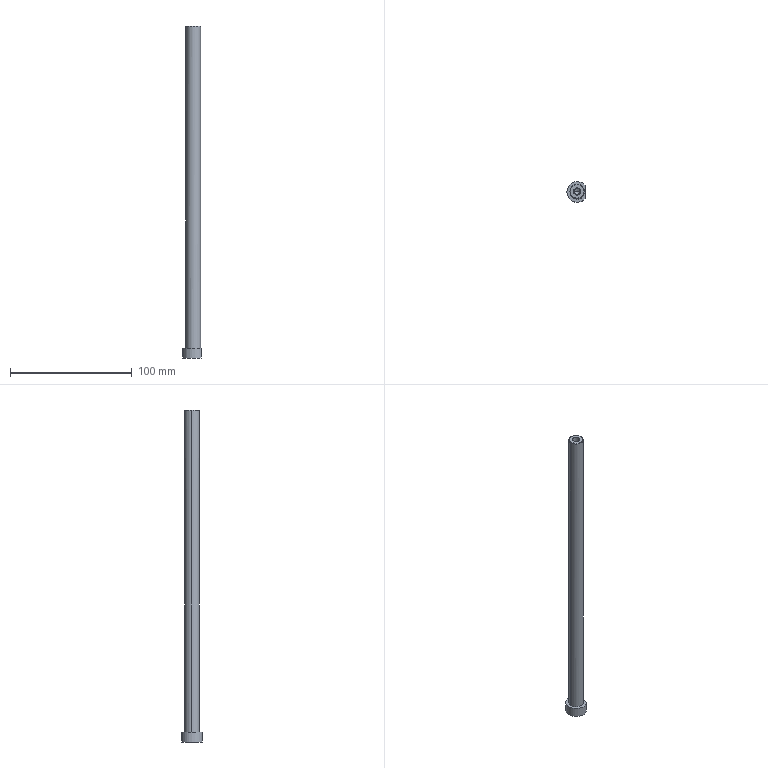Part | Creo | 1 solid | 16 faces | box 15 x 17 x 272.628 mm | volume 31426 mm3 | cylinder 7 | plane 5 | cone 4 | commonest cylinder face diameters 5 x2 6 x2 12 x2 17 x1
STEP:
#1=CARTESIAN_POINT('',(31.5,-23.477,-288.));
#2=VERTEX_POINT('',#1);
#3=CARTESIAN_POINT('',(31.5,-12.523,-288.));
#4=VERTEX_POINT('',#3);
#5=CARTESIAN_POINT('',(31.5,-23.477,-288.));
#6=DIRECTION('',(0.,1.,0.));
#7=VECTOR('',#6,10.954);
#8=LINE('',#5,#7);
#9=EDGE_CURVE('',#2,#4,#8,.T.);
#10=ORIENTED_EDGE('',*,*,#9,.F.);
#11=CARTESIAN_POINT('',(25.,-18.,-288.));
#12=DIRECTION('',(0.,0.,1.));
#13=DIRECTION('',(0.7647,0.6444,0.));
#14=AXIS2_PLACEMENT_3D('',#11,#12,#13);
#15=CIRCLE('',#14,8.5);
#16=EDGE_CURVE('',#4,#2,#15,.T.);
#17=ORIENTED_EDGE('',*,*,#16,.F.);
#18=EDGE_LOOP('',(#10,#17));
#19=FACE_OUTER_BOUND('',#18,.F.);
#20=CARTESIAN_POINT('',(19.,-18.,-288.));
#21=VERTEX_POINT('',#20);
#22=CARTESIAN_POINT('',(31.,-18.,-288.));
#23=VERTEX_POINT('',#22);
#24=CARTESIAN_POINT('',(25.,-18.,-288.));
#25=DIRECTION('',(0.,0.,-1.));
#26=DIRECTION('',(-1.,0.,0.));
#27=AXIS2_PLACEMENT_3D('',#24,#25,#26);
#28=CIRCLE('',#27,6.);
#29=EDGE_CURVE('',#21,#23,#28,.T.);
#30=ORIENTED_EDGE('',*,*,#29,.F.);
#31=CARTESIAN_POINT('',(25.,-18.,-288.));
#32=DIRECTION('',(0.,0.,-1.));
#33=DIRECTION('',(1.,0.,0.));
#34=AXIS2_PLACEMENT_3D('',#31,#32,#33);
#35=CIRCLE('',#34,6.);
#36=EDGE_CURVE('',#23,#21,#35,.T.);
#37=ORIENTED_EDGE('',*,*,#36,.F.);
#38=EDGE_LOOP('',(#30,#37));
#39=FACE_BOUND('',#38,.F.);
#40=CARTESIAN_POINT('',(25.,-18.,-288.));
#41=DIRECTION('',(0.,0.,1.));
#42=DIRECTION('',(-1.,0.,0.));
#43=AXIS2_PLACEMENT_3D('',#40,#41,#42);
#44=PLANE('',#43);
#45=ADVANCED_FACE('',(#19,#39),#44,.T.);
#46=CARTESIAN_POINT('',(31.5,-23.477,-296.));
#47=VERTEX_POINT('',#46);
#48=CARTESIAN_POINT('',(31.5,-23.477,-296.));
#49=DIRECTION('',(0.,0.,1.));
#50=VECTOR('',#49,8.);
#51=LINE('',#48,#50);
#52=EDGE_CURVE('',#47,#2,#51,.T.);
#53=ORIENTED_EDGE('',*,*,#52,.T.);
#54=ORIENTED_EDGE('',*,*,#9,.T.);
#55=CARTESIAN_POINT('',(31.5,-12.523,-296.));
#56=VERTEX_POINT('',#55);
#57=CARTESIAN_POINT('',(31.5,-12.523,-288.));
#58=DIRECTION('',(0.,0.,-1.));
#59=VECTOR('',#58,8.);
#60=LINE('',#57,#59);
#61=EDGE_CURVE('',#4,#56,#60,.T.);
#62=ORIENTED_EDGE('',*,*,#61,.T.);
#63=CARTESIAN_POINT('',(31.5,-12.523,-296.));
#64=DIRECTION('',(0.,-1.,0.));
#65=VECTOR('',#64,10.954);
#66=LINE('',#63,#65);
#67=EDGE_CURVE('',#56,#47,#66,.T.);
#68=ORIENTED_EDGE('',*,*,#67,.T.);
#69=EDGE_LOOP('',(#53,#54,#62,#68));
#70=FACE_OUTER_BOUND('',#69,.F.);
#71=CARTESIAN_POINT('',(31.5,17.,-297.));
#72=DIRECTION('',(-1.,0.,0.));
#73=DIRECTION('',(0.,0.,-1.));
#74=AXIS2_PLACEMENT_3D('',#71,#72,#73);
#75=PLANE('',#74);
#76=ADVANCED_FACE('',(#70),#75,.F.);
#77=ORIENTED_EDGE('',*,*,#52,.F.);
#78=CARTESIAN_POINT('',(25.,-18.,-296.));
#79=DIRECTION('',(0.,0.,-1.));
#80=DIRECTION('',(0.7647,-0.6444,0.));
#81=AXIS2_PLACEMENT_3D('',#78,#79,#80);
#82=CIRCLE('',#81,8.5);
#83=EDGE_CURVE('',#47,#56,#82,.T.);
#84=ORIENTED_EDGE('',*,*,#83,.T.);
#85=ORIENTED_EDGE('',*,*,#61,.F.);
#86=ORIENTED_EDGE('',*,*,#16,.T.);
#87=EDGE_LOOP('',(#77,#84,#85,#86));
#88=FACE_OUTER_BOUND('',#87,.F.);
#89=CARTESIAN_POINT('',(25.,-18.,-296.));
#90=DIRECTION('',(0.,0.,1.));
#91=DIRECTION('',(-1.,0.,0.));
#92=AXIS2_PLACEMENT_3D('',#89,#90,#91);
#93=CYLINDRICAL_SURFACE('',#92,8.5);
#94=ADVANCED_FACE('',(#88),#93,.T.);
#95=ORIENTED_EDGE('',*,*,#67,.F.);
#96=ORIENTED_EDGE('',*,*,#83,.F.);
#97=EDGE_LOOP('',(#95,#96));
#98=FACE_OUTER_BOUND('',#97,.F.);
#99=CARTESIAN_POINT('',(25.,-18.,-296.));
#100=DIRECTION('',(0.,0.,-1.));
#101=DIRECTION('',(1.,0.,0.));
#102=AXIS2_PLACEMENT_3D('',#99,#100,#101);
#103=PLANE('',#102);
#104=ADVANCED_FACE('',(#98),#103,.T.);
#105=ORIENTED_EDGE('',*,*,#29,.T.);
#106=CARTESIAN_POINT('',(31.,-18.,-23.872));
#107=VERTEX_POINT('',#106);
#108=CARTESIAN_POINT('',(31.,-18.,-288.));
#109=DIRECTION('',(0.,0.,1.));
#110=VECTOR('',#109,264.128);
#111=LINE('',#108,#110);
#112=EDGE_CURVE('',#23,#107,#111,.T.);
#113=ORIENTED_EDGE('',*,*,#112,.T.);
#114=CARTESIAN_POINT('',(25.,-12.,-23.872));
#115=VERTEX_POINT('',#114);
#116=CARTESIAN_POINT('',(25.,-18.,-23.872));
#117=DIRECTION('',(0.,0.,1.));
#118=DIRECTION('',(1.,0.,0.));
#119=AXIS2_PLACEMENT_3D('',#116,#117,#118);
#120=CIRCLE('',#119,6.);
#121=EDGE_CURVE('',#107,#115,#120,.T.);
#122=ORIENTED_EDGE('',*,*,#121,.T.);
#123=CARTESIAN_POINT('',(19.,-18.,-23.872));
#124=VERTEX_POINT('',#123);
#125=CARTESIAN_POINT('',(25.,-18.,-23.872));
#126=DIRECTION('',(0.,0.,1.));
#127=DIRECTION('',(0.,1.,0.));
#128=AXIS2_PLACEMENT_3D('',#125,#126,#127);
#129=CIRCLE('',#128,6.);
#130=EDGE_CURVE('',#115,#124,#129,.T.);
#131=ORIENTED_EDGE('',*,*,#130,.T.);
#132=CARTESIAN_POINT('',(19.,-18.,-288.));
#133=DIRECTION('',(0.,0.,1.));
#134=VECTOR('',#133,264.128);
#135=LINE('',#132,#134);
#136=EDGE_CURVE('',#21,#124,#135,.T.);
#137=ORIENTED_EDGE('',*,*,#136,.F.);
#138=EDGE_LOOP('',(#105,#113,#122,#131,#137));
#139=FACE_OUTER_BOUND('',#138,.F.);
#140=CARTESIAN_POINT('',(25.,-18.,-351.131));
#141=DIRECTION('',(0.,0.,1.));
#142=DIRECTION('',(-1.,0.,0.));
#143=AXIS2_PLACEMENT_3D('',#140,#141,#142);
#144=CYLINDRICAL_SURFACE('',#143,6.);
#145=ADVANCED_FACE('',(#139),#144,.T.);
#146=ORIENTED_EDGE('',*,*,#36,.T.);
#147=ORIENTED_EDGE('',*,*,#136,.T.);
#148=CARTESIAN_POINT('',(25.,-24.,-23.872));
#149=VERTEX_POINT('',#148);
#150=CARTESIAN_POINT('',(25.,-18.,-23.872));
#151=DIRECTION('',(0.,0.,1.));
#152=DIRECTION('',(-1.,0.,0.));
#153=AXIS2_PLACEMENT_3D('',#150,#151,#152);
#154=CIRCLE('',#153,6.);
#155=EDGE_CURVE('',#124,#149,#154,.T.);
#156=ORIENTED_EDGE('',*,*,#155,.T.);
#157=CARTESIAN_POINT('',(25.,-18.,-23.872));
#158=DIRECTION('',(0.,0.,1.));
#159=DIRECTION('',(0.,-1.,0.));
#160=AXIS2_PLACEMENT_3D('',#157,#158,#159);
#161=CIRCLE('',#160,6.);
#162=EDGE_CURVE('',#149,#107,#161,.T.);
#163=ORIENTED_EDGE('',*,*,#162,.T.);
#164=ORIENTED_EDGE('',*,*,#112,.F.);
#165=EDGE_LOOP('',(#146,#147,#156,#163,#164));
#166=FACE_OUTER_BOUND('',#165,.F.);
#167=CARTESIAN_POINT('',(25.,-18.,-351.131));
#168=DIRECTION('',(0.,0.,1.));
#169=DIRECTION('',(-1.,0.,0.));
#170=AXIS2_PLACEMENT_3D('',#167,#168,#169);
#171=CYLINDRICAL_SURFACE('',#170,6.);
#172=ADVANCED_FACE('',(#166),#171,.T.);
#173=CARTESIAN_POINT('',(25.,-12.5,-23.372));
#174=VERTEX_POINT('',#173);
#175=CARTESIAN_POINT('',(25.,-23.5,-23.372));
#176=VERTEX_POINT('',#175);
#177=CARTESIAN_POINT('',(25.,-18.,-23.372));
#178=DIRECTION('',(0.,0.,1.));
#179=DIRECTION('',(0.,1.,0.));
#180=AXIS2_PLACEMENT_3D('',#177,#178,#179);
#181=CIRCLE('',#180,5.5);
#182=EDGE_CURVE('',#174,#176,#181,.T.);
#183=ORIENTED_EDGE('',*,*,#182,.T.);
#184=CARTESIAN_POINT('',(25.,-23.5,-23.372));
#185=DIRECTION('',(0.,-0.7071,-0.7071));
#186=VECTOR('',#185,0.7071);
#187=LINE('',#184,#186);
#188=EDGE_CURVE('',#176,#149,#187,.T.);
#189=ORIENTED_EDGE('',*,*,#188,.T.);
#190=ORIENTED_EDGE('',*,*,#155,.F.);
#191=ORIENTED_EDGE('',*,*,#130,.F.);
#192=CARTESIAN_POINT('',(25.,-12.5,-23.372));
#193=DIRECTION('',(0.,0.7071,-0.7071));
#194=VECTOR('',#193,0.7071);
#195=LINE('',#192,#194);
#196=EDGE_CURVE('',#174,#115,#195,.T.);
#197=ORIENTED_EDGE('',*,*,#196,.F.);
#198=EDGE_LOOP('',(#183,#189,#190,#191,#197));
#199=FACE_OUTER_BOUND('',#198,.F.);
#200=CARTESIAN_POINT('',(25.,-18.,-23.622));
#201=DIRECTION('',(0.,0.,-1.));
#202=DIRECTION('',(0.,-1.,0.));
#203=AXIS2_PLACEMENT_3D('',#200,#201,#202);
#204=CONICAL_SURFACE('',#203,5.75,45.);
#205=ADVANCED_FACE('',(#199),#204,.T.);
#206=ORIENTED_EDGE('',*,*,#182,.F.);
#207=CARTESIAN_POINT('',(25.,-18.,-23.372));
#208=DIRECTION('',(0.,0.,1.));
#209=DIRECTION('',(0.,-1.,0.));
#210=AXIS2_PLACEMENT_3D('',#207,#208,#209);
#211=CIRCLE('',#210,5.5);
#212=EDGE_CURVE('',#176,#174,#211,.T.);
#213=ORIENTED_EDGE('',*,*,#212,.F.);
#214=EDGE_LOOP('',(#206,#213));
#215=FACE_OUTER_BOUND('',#214,.F.);
#216=CARTESIAN_POINT('',(28.,-18.,-23.372));
#217=VERTEX_POINT('',#216);
#218=CARTESIAN_POINT('',(22.,-18.,-23.372));
#219=VERTEX_POINT('',#218);
#220=CARTESIAN_POINT('',(25.,-18.,-23.372));
#221=DIRECTION('',(0.,0.,-1.));
#222=DIRECTION('',(1.,0.,0.));
#223=AXIS2_PLACEMENT_3D('',#220,#221,#222);
#224=CIRCLE('',#223,3.);
#225=EDGE_CURVE('',#217,#219,#224,.T.);
#226=ORIENTED_EDGE('',*,*,#225,.F.);
#227=CARTESIAN_POINT('',(25.,-18.,-23.372));
#228=DIRECTION('',(0.,0.,-1.));
#229=DIRECTION('',(-1.,0.,0.));
#230=AXIS2_PLACEMENT_3D('',#227,#228,#229);
#231=CIRCLE('',#230,3.);
#232=EDGE_CURVE('',#219,#217,#231,.T.);
#233=ORIENTED_EDGE('',*,*,#232,.F.);
#234=EDGE_LOOP('',(#226,#233));
#235=FACE_BOUND('',#234,.F.);
#236=CARTESIAN_POINT('',(25.,-14.7,-23.372));
#237=DIRECTION('',(0.,0.,-1.));
#238=DIRECTION('',(1.,0.,0.));
#239=AXIS2_PLACEMENT_3D('',#236,#237,#238);
#240=PLANE('',#239);
#241=ADVANCED_FACE('',(#215,#235),#240,.F.);
#242=ORIENTED_EDGE('',*,*,#212,.T.);
#243=ORIENTED_EDGE('',*,*,#196,.T.);
#244=ORIENTED_EDGE('',*,*,#121,.F.);
#245=ORIENTED_EDGE('',*,*,#162,.F.);
#246=ORIENTED_EDGE('',*,*,#188,.F.);
#247=EDGE_LOOP('',(#242,#243,#244,#245,#246));
#248=FACE_OUTER_BOUND('',#247,.F.);
#249=CARTESIAN_POINT('',(25.,-18.,-23.622));
#250=DIRECTION('',(0.,0.,-1.));
#251=DIRECTION('',(0.,-1.,0.));
#252=AXIS2_PLACEMENT_3D('',#249,#250,#251);
#253=CONICAL_SURFACE('',#252,5.75,45.);
#254=ADVANCED_FACE('',(#248),#253,.T.);
#255=CARTESIAN_POINT('',(22.,-18.,-28.872));
#256=VERTEX_POINT('',#255);
#257=CARTESIAN_POINT('',(28.,-18.,-28.872));
#258=VERTEX_POINT('',#257);
#259=CARTESIAN_POINT('',(25.,-18.,-28.872));
#260=DIRECTION('',(0.,0.,1.));
#261=DIRECTION('',(-1.,0.,0.));
#262=AXIS2_PLACEMENT_3D('',#259,#260,#261);
#263=CIRCLE('',#262,3.);
#264=EDGE_CURVE('',#256,#258,#263,.T.);
#265=ORIENTED_EDGE('',*,*,#264,.T.);
#266=CARTESIAN_POINT('',(28.,-18.,-23.372));
#267=DIRECTION('',(0.,0.,-1.));
#268=VECTOR('',#267,5.5);
#269=LINE('',#266,#268);
#270=EDGE_CURVE('',#217,#258,#269,.T.);
#271=ORIENTED_EDGE('',*,*,#270,.F.);
#272=ORIENTED_EDGE('',*,*,#225,.T.);
#273=CARTESIAN_POINT('',(22.,-18.,-23.372));
#274=DIRECTION('',(0.,0.,-1.));
#275=VECTOR('',#274,5.5);
#276=LINE('',#273,#275);
#277=EDGE_CURVE('',#219,#256,#276,.T.);
#278=ORIENTED_EDGE('',*,*,#277,.T.);
#279=EDGE_LOOP('',(#265,#271,#272,#278));
#280=FACE_OUTER_BOUND('',#279,.F.);
#281=CARTESIAN_POINT('',(25.,-18.,-6.372));
#282=DIRECTION('',(0.,0.,-1.));
#283=DIRECTION('',(1.,0.,0.));
#284=AXIS2_PLACEMENT_3D('',#281,#282,#283);
#285=CYLINDRICAL_SURFACE('',#284,3.);
#286=ADVANCED_FACE('',(#280),#285,.F.);
#287=CARTESIAN_POINT('',(25.,-18.,-28.872));
#288=DIRECTION('',(0.,0.,1.));
#289=DIRECTION('',(1.,0.,0.));
#290=AXIS2_PLACEMENT_3D('',#287,#288,#289);
#291=CIRCLE('',#290,3.);
#292=EDGE_CURVE('',#258,#256,#291,.T.);
#293=ORIENTED_EDGE('',*,*,#292,.F.);
#294=ORIENTED_EDGE('',*,*,#264,.F.);
#295=EDGE_LOOP('',(#293,#294));
#296=FACE_OUTER_BOUND('',#295,.F.);
#297=CARTESIAN_POINT('',(27.5,-18.,-28.872));
#298=VERTEX_POINT('',#297);
#299=CARTESIAN_POINT('',(22.5,-18.,-28.872));
#300=VERTEX_POINT('',#299);
#301=CARTESIAN_POINT('',(25.,-18.,-28.872));
#302=DIRECTION('',(0.,0.,-1.));
#303=DIRECTION('',(1.,0.,0.));
#304=AXIS2_PLACEMENT_3D('',#301,#302,#303);
#305=CIRCLE('',#304,2.5);
#306=EDGE_CURVE('',#298,#300,#305,.T.);
#307=ORIENTED_EDGE('',*,*,#306,.F.);
#308=CARTESIAN_POINT('',(25.,-18.,-28.872));
#309=DIRECTION('',(0.,0.,-1.));
#310=DIRECTION('',(-1.,0.,0.));
#311=AXIS2_PLACEMENT_3D('',#308,#309,#310);
#312=CIRCLE('',#311,2.5);
#313=EDGE_CURVE('',#300,#298,#312,.T.);
#314=ORIENTED_EDGE('',*,*,#313,.F.);
#315=EDGE_LOOP('',(#307,#314));
#316=FACE_BOUND('',#315,.F.);
#317=CARTESIAN_POINT('',(25.,-18.,-28.872));
#318=DIRECTION('',(0.,0.,-1.));
#319=DIRECTION('',(1.,0.,0.));
#320=AXIS2_PLACEMENT_3D('',#317,#318,#319);
#321=PLANE('',#320);
#322=ADVANCED_FACE('',(#296,#316),#321,.F.);
#323=ORIENTED_EDGE('',*,*,#306,.T.);
#324=CARTESIAN_POINT('',(22.5,-18.,-30.342));
#325=VERTEX_POINT('',#324);
#326=CARTESIAN_POINT('',(22.5,-18.,-28.872));
#327=DIRECTION('',(0.,0.,-1.));
#328=VECTOR('',#327,1.47);
#329=LINE('',#326,#328);
#330=EDGE_CURVE('',#300,#325,#329,.T.);
#331=ORIENTED_EDGE('',*,*,#330,.T.);
#332=CARTESIAN_POINT('',(27.5,-18.,-30.342));
#333=VERTEX_POINT('',#332);
#334=CARTESIAN_POINT('',(25.,-18.,-30.342));
#335=DIRECTION('',(0.,0.,1.));
#336=DIRECTION('',(-1.,0.,0.));
#337=AXIS2_PLACEMENT_3D('',#334,#335,#336);
#338=CIRCLE('',#337,2.5);
#339=EDGE_CURVE('',#325,#333,#338,.T.);
#340=ORIENTED_EDGE('',*,*,#339,.T.);
#341=CARTESIAN_POINT('',(27.5,-18.,-28.872));
#342=DIRECTION('',(0.,0.,-1.));
#343=VECTOR('',#342,1.47);
#344=LINE('',#341,#343);
#345=EDGE_CURVE('',#298,#333,#344,.T.);
#346=ORIENTED_EDGE('',*,*,#345,.F.);
#347=EDGE_LOOP('',(#323,#331,#340,#346));
#348=FACE_OUTER_BOUND('',#347,.F.);
#349=CARTESIAN_POINT('',(25.,-18.,-6.372));
#350=DIRECTION('',(0.,0.,-1.));
#351=DIRECTION('',(1.,0.,0.));
#352=AXIS2_PLACEMENT_3D('',#349,#350,#351);
#353=CYLINDRICAL_SURFACE('',#352,2.5);
#354=ADVANCED_FACE('',(#348),#353,.F.);
#355=ORIENTED_EDGE('',*,*,#313,.T.);
#356=ORIENTED_EDGE('',*,*,#345,.T.);
#357=CARTESIAN_POINT('',(25.,-15.5,-30.342));
#358=VERTEX_POINT('',#357);
#359=CARTESIAN_POINT('',(25.,-18.,-30.342));
#360=DIRECTION('',(0.,0.,1.));
#361=DIRECTION('',(1.,0.,0.));
#362=AXIS2_PLACEMENT_3D('',#359,#360,#361);
#363=CIRCLE('',#362,2.5);
#364=EDGE_CURVE('',#333,#358,#363,.T.);
#365=ORIENTED_EDGE('',*,*,#364,.T.);
#366=CARTESIAN_POINT('',(25.,-18.,-30.342));
#367=DIRECTION('',(0.,0.,1.));
#368=DIRECTION('',(0.,1.,0.));
#369=AXIS2_PLACEMENT_3D('',#366,#367,#368);
#370=CIRCLE('',#369,2.5);
#371=EDGE_CURVE('',#358,#325,#370,.T.);
#372=ORIENTED_EDGE('',*,*,#371,.T.);
#373=ORIENTED_EDGE('',*,*,#330,.F.);
#374=EDGE_LOOP('',(#355,#356,#365,#372,#373));
#375=FACE_OUTER_BOUND('',#374,.F.);
#376=CARTESIAN_POINT('',(25.,-18.,-6.372));
#377=DIRECTION('',(0.,0.,-1.));
#378=DIRECTION('',(1.,0.,0.));
#379=AXIS2_PLACEMENT_3D('',#376,#377,#378);
#380=CYLINDRICAL_SURFACE('',#379,2.5);
#381=ADVANCED_FACE('',(#375),#380,.F.);
#382=ORIENTED_EDGE('',*,*,#371,.F.);
#383=ORIENTED_EDGE('',*,*,#364,.F.);
#384=CARTESIAN_POINT('',(25.,-18.,-31.844));
#385=VERTEX_POINT('',#384);
#386=CARTESIAN_POINT('',(25.,-18.,-31.844));
#387=DIRECTION('',(0.8572,0.,0.515));
#388=VECTOR('',#387,2.917);
#389=LINE('',#386,#388);
#390=EDGE_CURVE('',#385,#333,#389,.T.);
#391=ORIENTED_EDGE('',*,*,#390,.F.);
#392=CARTESIAN_POINT('',(25.,-18.,-31.844));
#393=DIRECTION('',(-0.8572,0.,0.515));
#394=VECTOR('',#393,2.917);
#395=LINE('',#392,#394);
#396=EDGE_CURVE('',#385,#325,#395,.T.);
#397=ORIENTED_EDGE('',*,*,#396,.T.);
#398=EDGE_LOOP('',(#382,#383,#391,#397));
#399=FACE_OUTER_BOUND('',#398,.F.);
#400=CARTESIAN_POINT('',(25.,-18.,-31.008));
#401=DIRECTION('',(0.,0.,1.));
#402=DIRECTION('',(1.,0.,0.));
#403=AXIS2_PLACEMENT_3D('',#400,#401,#402);
#404=CONICAL_SURFACE('',#403,1.391,59.);
#405=ADVANCED_FACE('',(#399),#404,.F.);
#406=ORIENTED_EDGE('',*,*,#339,.F.);
#407=ORIENTED_EDGE('',*,*,#396,.F.);
#408=ORIENTED_EDGE('',*,*,#390,.T.);
#409=EDGE_LOOP('',(#406,#407,#408));
#410=FACE_OUTER_BOUND('',#409,.F.);
#411=CARTESIAN_POINT('',(25.,-18.,-31.008));
#412=DIRECTION('',(0.,0.,1.));
#413=DIRECTION('',(1.,0.,0.));
#414=AXIS2_PLACEMENT_3D('',#411,#412,#413);
#415=CONICAL_SURFACE('',#414,1.391,59.);
#416=ADVANCED_FACE('',(#410),#415,.F.);
#417=ORIENTED_EDGE('',*,*,#292,.T.);
#418=ORIENTED_EDGE('',*,*,#277,.F.);
#419=ORIENTED_EDGE('',*,*,#232,.T.);
#420=ORIENTED_EDGE('',*,*,#270,.T.);
#421=EDGE_LOOP('',(#417,#418,#419,#420));
#422=FACE_OUTER_BOUND('',#421,.F.);
#423=CARTESIAN_POINT('',(25.,-18.,-6.372));
#424=DIRECTION('',(0.,0.,-1.));
#425=DIRECTION('',(1.,0.,0.));
#426=AXIS2_PLACEMENT_3D('',#423,#424,#425);
#427=CYLINDRICAL_SURFACE('',#426,3.);
#428=ADVANCED_FACE('',(#422),#427,.F.);
#429=CLOSED_SHELL('',(#45,#76,#94,#104,#145,#172,#205,#241,#254,#286,#322,#354,#381,#405,#416,#428));
#430=MANIFOLD_SOLID_BREP('',#429);
#431=(LENGTH_UNIT()NAMED_UNIT(*)SI_UNIT(.MILLI.,.METRE.));
#432=UNCERTAINTY_MEASURE_WITH_UNIT(LENGTH_MEASURE(0.02736),#431,'','');
#433=(NAMED_UNIT(*)PLANE_ANGLE_UNIT()SI_UNIT($,.RADIAN.));
#434=PLANE_ANGLE_MEASURE_WITH_UNIT(PLANE_ANGLE_MEASURE(0.01745),#433);
#435=(CONVERSION_BASED_UNIT('DEGREE',#434)NAMED_UNIT(*)PLANE_ANGLE_UNIT());
#436=(NAMED_UNIT(*)SI_UNIT($,.STERADIAN.)SOLID_ANGLE_UNIT());
#437=(GEOMETRIC_REPRESENTATION_CONTEXT(3)GLOBAL_UNCERTAINTY_ASSIGNED_CONTEXT((#432))GLOBAL_UNIT_ASSIGNED_CONTEXT((#431,#435,#436))REPRESENTATION_CONTEXT('',''));
#438=ADVANCED_BREP_SHAPE_REPRESENTATION('',(#430),#437);